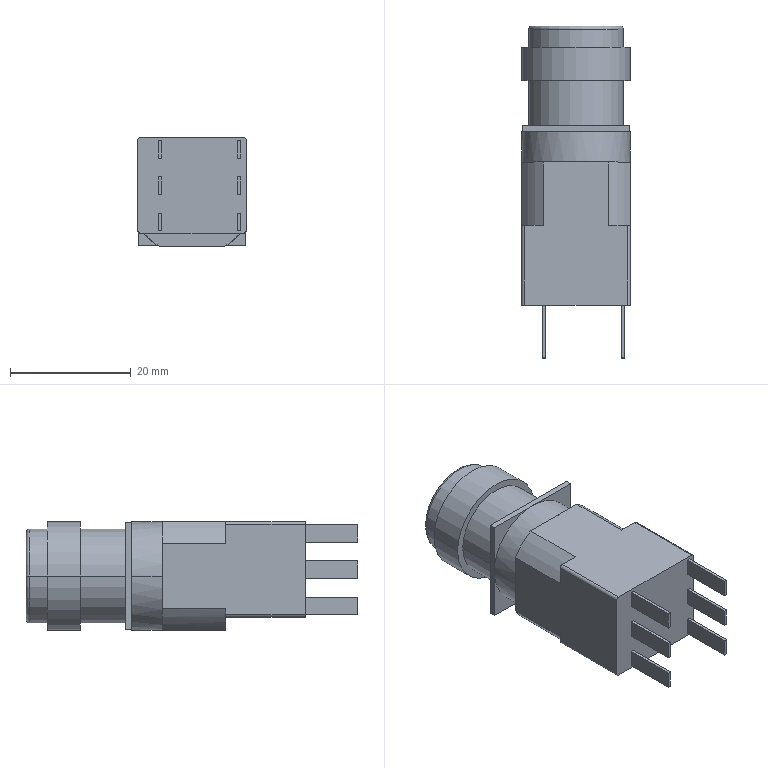Part | NX | 1 solid | 76 faces | box 18 x 54.9 x 18 mm | volume 12077 mm3 | plane 58 | cylinder 16 | torus 2 | commonest cylinder face diameters 1 x4 15.6 x4 21 x4 17.9 x2 18 x2